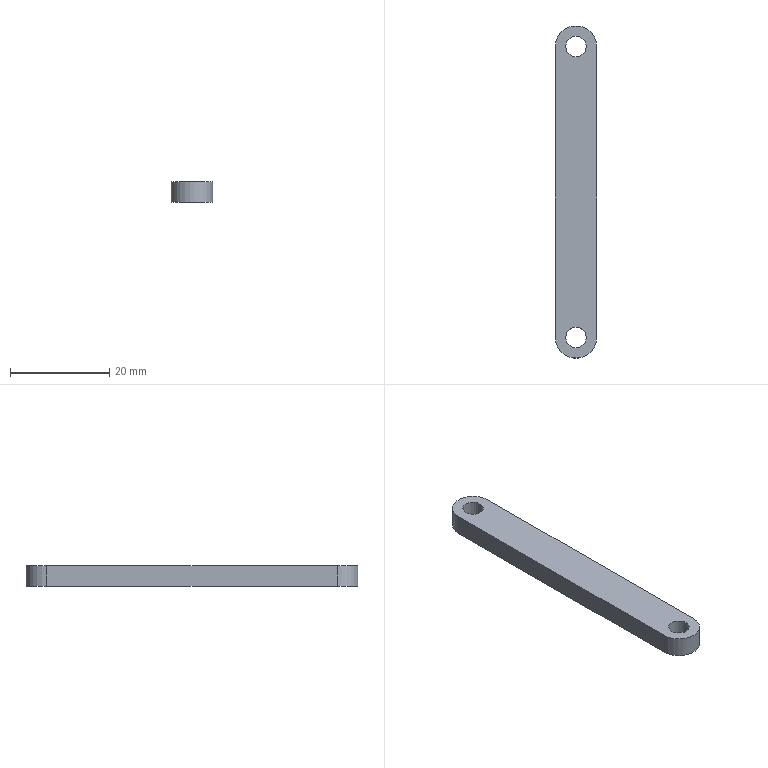Part | SolidWorks | features Extrusion 1, Scale 1 | 1 solid | 10 faces | box 8.32 x 66.82 x 4.134 mm | volume 2126 mm3 | cylinder 6 | plane 4 | commonest cylinder face diameters 4.134 x4 8.32 x2
STEP:
#1=CARTESIAN_POINT('',(-2.067,58.5,4.134));
#2=VERTEX_POINT('',#1);
#3=CARTESIAN_POINT('',(2.067,58.5,4.134));
#4=VERTEX_POINT('',#3);
#5=CARTESIAN_POINT('',(0.,58.5,4.134));
#6=DIRECTION('',(0.,0.,1.));
#7=DIRECTION('',(1.,0.,0.));
#8=AXIS2_PLACEMENT_3D('',#5,#6,#7);
#9=CIRCLE('',#8,2.067);
#10=EDGE_CURVE('',#2,#4,#9,.T.);
#11=ORIENTED_EDGE('',*,*,#10,.T.);
#12=CARTESIAN_POINT('',(2.067,58.5,0.));
#13=VERTEX_POINT('',#12);
#14=CARTESIAN_POINT('',(2.067,58.5,4.134));
#15=DIRECTION('',(0.,0.,-1.));
#16=VECTOR('',#15,1000.);
#17=LINE('',#14,#16);
#18=EDGE_CURVE('',#4,#13,#17,.T.);
#19=ORIENTED_EDGE('',*,*,#18,.T.);
#20=CARTESIAN_POINT('',(-2.067,58.5,0.));
#21=VERTEX_POINT('',#20);
#22=CARTESIAN_POINT('',(0.,58.5,0.));
#23=DIRECTION('',(0.,0.,1.));
#24=DIRECTION('',(1.,0.,0.));
#25=AXIS2_PLACEMENT_3D('',#22,#23,#24);
#26=CIRCLE('',#25,2.067);
#27=EDGE_CURVE('',#21,#13,#26,.T.);
#28=ORIENTED_EDGE('',*,*,#27,.F.);
#29=CARTESIAN_POINT('',(-2.067,58.5,4.134));
#30=DIRECTION('',(0.,0.,-1.));
#31=VECTOR('',#30,1000.);
#32=LINE('',#29,#31);
#33=EDGE_CURVE('',#2,#21,#32,.T.);
#34=ORIENTED_EDGE('',*,*,#33,.F.);
#35=EDGE_LOOP('',(#11,#19,#28,#34));
#36=FACE_OUTER_BOUND('',#35,.T.);
#37=CARTESIAN_POINT('',(0.,58.5,4.134));
#38=DIRECTION('',(0.,0.,-1.));
#39=DIRECTION('',(-1.,0.,0.));
#40=AXIS2_PLACEMENT_3D('',#37,#38,#39);
#41=CYLINDRICAL_SURFACE('',#40,2.067);
#42=ADVANCED_FACE('',(#36),#41,.F.);
#43=CARTESIAN_POINT('',(-2.067,0.,4.134));
#44=VERTEX_POINT('',#43);
#45=CARTESIAN_POINT('',(2.067,0.,4.134));
#46=VERTEX_POINT('',#45);
#47=CARTESIAN_POINT('',(0.,0.,4.134));
#48=DIRECTION('',(0.,0.,1.));
#49=DIRECTION('',(1.,0.,0.));
#50=AXIS2_PLACEMENT_3D('',#47,#48,#49);
#51=CIRCLE('',#50,2.067);
#52=EDGE_CURVE('',#44,#46,#51,.T.);
#53=ORIENTED_EDGE('',*,*,#52,.T.);
#54=CARTESIAN_POINT('',(2.067,0.,0.));
#55=VERTEX_POINT('',#54);
#56=CARTESIAN_POINT('',(2.067,0.,4.134));
#57=DIRECTION('',(0.,0.,-1.));
#58=VECTOR('',#57,1000.);
#59=LINE('',#56,#58);
#60=EDGE_CURVE('',#46,#55,#59,.T.);
#61=ORIENTED_EDGE('',*,*,#60,.T.);
#62=CARTESIAN_POINT('',(-2.067,0.,0.));
#63=VERTEX_POINT('',#62);
#64=CARTESIAN_POINT('',(0.,0.,0.));
#65=DIRECTION('',(0.,0.,1.));
#66=DIRECTION('',(1.,0.,0.));
#67=AXIS2_PLACEMENT_3D('',#64,#65,#66);
#68=CIRCLE('',#67,2.067);
#69=EDGE_CURVE('',#63,#55,#68,.T.);
#70=ORIENTED_EDGE('',*,*,#69,.F.);
#71=CARTESIAN_POINT('',(-2.067,0.,4.134));
#72=DIRECTION('',(0.,0.,-1.));
#73=VECTOR('',#72,1000.);
#74=LINE('',#71,#73);
#75=EDGE_CURVE('',#44,#63,#74,.T.);
#76=ORIENTED_EDGE('',*,*,#75,.F.);
#77=EDGE_LOOP('',(#53,#61,#70,#76));
#78=FACE_OUTER_BOUND('',#77,.T.);
#79=CARTESIAN_POINT('',(0.,0.,4.134));
#80=DIRECTION('',(0.,0.,-1.));
#81=DIRECTION('',(-1.,0.,0.));
#82=AXIS2_PLACEMENT_3D('',#79,#80,#81);
#83=CYLINDRICAL_SURFACE('',#82,2.067);
#84=ADVANCED_FACE('',(#78),#83,.F.);
#85=ORIENTED_EDGE('',*,*,#52,.F.);
#86=CARTESIAN_POINT('',(0.,0.,4.134));
#87=DIRECTION('',(0.,0.,1.));
#88=DIRECTION('',(1.,0.,0.));
#89=AXIS2_PLACEMENT_3D('',#86,#87,#88);
#90=CIRCLE('',#89,2.067);
#91=EDGE_CURVE('',#46,#44,#90,.T.);
#92=ORIENTED_EDGE('',*,*,#91,.F.);
#93=EDGE_LOOP('',(#85,#92));
#94=FACE_BOUND('',#93,.T.);
#95=CARTESIAN_POINT('',(-4.16,0.,4.134));
#96=VERTEX_POINT('',#95);
#97=CARTESIAN_POINT('',(4.16,0.,4.134));
#98=VERTEX_POINT('',#97);
#99=CARTESIAN_POINT('',(0.,0.,4.134));
#100=DIRECTION('',(0.,0.,1.));
#101=DIRECTION('',(1.,0.,0.));
#102=AXIS2_PLACEMENT_3D('',#99,#100,#101);
#103=CIRCLE('',#102,4.16);
#104=EDGE_CURVE('',#96,#98,#103,.T.);
#105=ORIENTED_EDGE('',*,*,#104,.T.);
#106=CARTESIAN_POINT('',(4.16,58.5,4.134));
#107=VERTEX_POINT('',#106);
#108=CARTESIAN_POINT('',(4.16,0.,4.134));
#109=DIRECTION('',(0.,1.,0.));
#110=VECTOR('',#109,1000.);
#111=LINE('',#108,#110);
#112=EDGE_CURVE('',#98,#107,#111,.T.);
#113=ORIENTED_EDGE('',*,*,#112,.T.);
#114=CARTESIAN_POINT('',(-4.16,58.5,4.134));
#115=VERTEX_POINT('',#114);
#116=CARTESIAN_POINT('',(0.,58.5,4.134));
#117=DIRECTION('',(0.,0.,1.));
#118=DIRECTION('',(1.,0.,0.));
#119=AXIS2_PLACEMENT_3D('',#116,#117,#118);
#120=CIRCLE('',#119,4.16);
#121=EDGE_CURVE('',#107,#115,#120,.T.);
#122=ORIENTED_EDGE('',*,*,#121,.T.);
#123=CARTESIAN_POINT('',(-4.16,0.,4.134));
#124=DIRECTION('',(0.,-1.,0.));
#125=VECTOR('',#124,1000.);
#126=LINE('',#123,#125);
#127=EDGE_CURVE('',#115,#96,#126,.T.);
#128=ORIENTED_EDGE('',*,*,#127,.T.);
#129=EDGE_LOOP('',(#105,#113,#122,#128));
#130=FACE_OUTER_BOUND('',#129,.T.);
#131=ORIENTED_EDGE('',*,*,#10,.F.);
#132=CARTESIAN_POINT('',(0.,58.5,4.134));
#133=DIRECTION('',(0.,0.,1.));
#134=DIRECTION('',(1.,0.,0.));
#135=AXIS2_PLACEMENT_3D('',#132,#133,#134);
#136=CIRCLE('',#135,2.067);
#137=EDGE_CURVE('',#4,#2,#136,.T.);
#138=ORIENTED_EDGE('',*,*,#137,.F.);
#139=EDGE_LOOP('',(#131,#138));
#140=FACE_BOUND('',#139,.T.);
#141=CARTESIAN_POINT('',(0.,0.,4.134));
#142=DIRECTION('',(0.,0.,1.));
#143=DIRECTION('',(1.,0.,0.));
#144=AXIS2_PLACEMENT_3D('',#141,#142,#143);
#145=PLANE('',#144);
#146=ADVANCED_FACE('',(#94,#130,#140),#145,.T.);
#147=CARTESIAN_POINT('',(-4.16,0.,0.));
#148=VERTEX_POINT('',#147);
#149=CARTESIAN_POINT('',(4.16,0.,0.));
#150=VERTEX_POINT('',#149);
#151=CARTESIAN_POINT('',(0.,0.,0.));
#152=DIRECTION('',(0.,0.,1.));
#153=DIRECTION('',(1.,0.,0.));
#154=AXIS2_PLACEMENT_3D('',#151,#152,#153);
#155=CIRCLE('',#154,4.16);
#156=EDGE_CURVE('',#148,#150,#155,.T.);
#157=ORIENTED_EDGE('',*,*,#156,.F.);
#158=CARTESIAN_POINT('',(-4.16,58.5,0.));
#159=VERTEX_POINT('',#158);
#160=CARTESIAN_POINT('',(-4.16,0.,0.));
#161=DIRECTION('',(0.,-1.,0.));
#162=VECTOR('',#161,1000.);
#163=LINE('',#160,#162);
#164=EDGE_CURVE('',#159,#148,#163,.T.);
#165=ORIENTED_EDGE('',*,*,#164,.F.);
#166=CARTESIAN_POINT('',(4.16,58.5,0.));
#167=VERTEX_POINT('',#166);
#168=CARTESIAN_POINT('',(0.,58.5,0.));
#169=DIRECTION('',(0.,0.,1.));
#170=DIRECTION('',(1.,0.,0.));
#171=AXIS2_PLACEMENT_3D('',#168,#169,#170);
#172=CIRCLE('',#171,4.16);
#173=EDGE_CURVE('',#167,#159,#172,.T.);
#174=ORIENTED_EDGE('',*,*,#173,.F.);
#175=CARTESIAN_POINT('',(4.16,0.,0.));
#176=DIRECTION('',(0.,1.,0.));
#177=VECTOR('',#176,1000.);
#178=LINE('',#175,#177);
#179=EDGE_CURVE('',#150,#167,#178,.T.);
#180=ORIENTED_EDGE('',*,*,#179,.F.);
#181=EDGE_LOOP('',(#157,#165,#174,#180));
#182=FACE_OUTER_BOUND('',#181,.T.);
#183=ORIENTED_EDGE('',*,*,#69,.T.);
#184=CARTESIAN_POINT('',(0.,0.,0.));
#185=DIRECTION('',(0.,0.,1.));
#186=DIRECTION('',(1.,0.,0.));
#187=AXIS2_PLACEMENT_3D('',#184,#185,#186);
#188=CIRCLE('',#187,2.067);
#189=EDGE_CURVE('',#55,#63,#188,.T.);
#190=ORIENTED_EDGE('',*,*,#189,.T.);
#191=EDGE_LOOP('',(#183,#190));
#192=FACE_BOUND('',#191,.T.);
#193=ORIENTED_EDGE('',*,*,#27,.T.);
#194=CARTESIAN_POINT('',(0.,58.5,0.));
#195=DIRECTION('',(0.,0.,1.));
#196=DIRECTION('',(1.,0.,0.));
#197=AXIS2_PLACEMENT_3D('',#194,#195,#196);
#198=CIRCLE('',#197,2.067);
#199=EDGE_CURVE('',#13,#21,#198,.T.);
#200=ORIENTED_EDGE('',*,*,#199,.T.);
#201=EDGE_LOOP('',(#193,#200));
#202=FACE_BOUND('',#201,.T.);
#203=CARTESIAN_POINT('',(0.,0.,0.));
#204=DIRECTION('',(0.,0.,1.));
#205=DIRECTION('',(1.,0.,0.));
#206=AXIS2_PLACEMENT_3D('',#203,#204,#205);
#207=PLANE('',#206);
#208=ADVANCED_FACE('',(#182,#192,#202),#207,.F.);
#209=ORIENTED_EDGE('',*,*,#156,.T.);
#210=CARTESIAN_POINT('',(4.16,0.,4.134));
#211=DIRECTION('',(0.,0.,-1.));
#212=VECTOR('',#211,1000.);
#213=LINE('',#210,#212);
#214=EDGE_CURVE('',#98,#150,#213,.T.);
#215=ORIENTED_EDGE('',*,*,#214,.F.);
#216=ORIENTED_EDGE('',*,*,#104,.F.);
#217=CARTESIAN_POINT('',(-4.16,0.,4.134));
#218=DIRECTION('',(0.,0.,-1.));
#219=VECTOR('',#218,1000.);
#220=LINE('',#217,#219);
#221=EDGE_CURVE('',#96,#148,#220,.T.);
#222=ORIENTED_EDGE('',*,*,#221,.T.);
#223=EDGE_LOOP('',(#209,#215,#216,#222));
#224=FACE_OUTER_BOUND('',#223,.T.);
#225=CARTESIAN_POINT('',(0.,0.,4.134));
#226=DIRECTION('',(0.,0.,-1.));
#227=DIRECTION('',(-1.,0.,0.));
#228=AXIS2_PLACEMENT_3D('',#225,#226,#227);
#229=CYLINDRICAL_SURFACE('',#228,4.16);
#230=ADVANCED_FACE('',(#224),#229,.T.);
#231=ORIENTED_EDGE('',*,*,#179,.T.);
#232=CARTESIAN_POINT('',(4.16,58.5,4.134));
#233=DIRECTION('',(0.,0.,-1.));
#234=VECTOR('',#233,1000.);
#235=LINE('',#232,#234);
#236=EDGE_CURVE('',#107,#167,#235,.T.);
#237=ORIENTED_EDGE('',*,*,#236,.F.);
#238=ORIENTED_EDGE('',*,*,#112,.F.);
#239=ORIENTED_EDGE('',*,*,#214,.T.);
#240=EDGE_LOOP('',(#231,#237,#238,#239));
#241=FACE_OUTER_BOUND('',#240,.T.);
#242=CARTESIAN_POINT('',(4.16,0.,4.134));
#243=DIRECTION('',(-1.,0.,0.));
#244=DIRECTION('',(0.,0.,1.));
#245=AXIS2_PLACEMENT_3D('',#242,#243,#244);
#246=PLANE('',#245);
#247=ADVANCED_FACE('',(#241),#246,.F.);
#248=ORIENTED_EDGE('',*,*,#173,.T.);
#249=CARTESIAN_POINT('',(-4.16,58.5,4.134));
#250=DIRECTION('',(0.,0.,-1.));
#251=VECTOR('',#250,1000.);
#252=LINE('',#249,#251);
#253=EDGE_CURVE('',#115,#159,#252,.T.);
#254=ORIENTED_EDGE('',*,*,#253,.F.);
#255=ORIENTED_EDGE('',*,*,#121,.F.);
#256=ORIENTED_EDGE('',*,*,#236,.T.);
#257=EDGE_LOOP('',(#248,#254,#255,#256));
#258=FACE_OUTER_BOUND('',#257,.T.);
#259=CARTESIAN_POINT('',(0.,58.5,4.134));
#260=DIRECTION('',(0.,0.,-1.));
#261=DIRECTION('',(-1.,0.,0.));
#262=AXIS2_PLACEMENT_3D('',#259,#260,#261);
#263=CYLINDRICAL_SURFACE('',#262,4.16);
#264=ADVANCED_FACE('',(#258),#263,.T.);
#265=ORIENTED_EDGE('',*,*,#164,.T.);
#266=ORIENTED_EDGE('',*,*,#221,.F.);
#267=ORIENTED_EDGE('',*,*,#127,.F.);
#268=ORIENTED_EDGE('',*,*,#253,.T.);
#269=EDGE_LOOP('',(#265,#266,#267,#268));
#270=FACE_OUTER_BOUND('',#269,.T.);
#271=CARTESIAN_POINT('',(-4.16,0.,4.134));
#272=DIRECTION('',(1.,0.,0.));
#273=DIRECTION('',(0.,0.,-1.));
#274=AXIS2_PLACEMENT_3D('',#271,#272,#273);
#275=PLANE('',#274);
#276=ADVANCED_FACE('',(#270),#275,.F.);
#277=ORIENTED_EDGE('',*,*,#60,.F.);
#278=ORIENTED_EDGE('',*,*,#91,.T.);
#279=ORIENTED_EDGE('',*,*,#75,.T.);
#280=ORIENTED_EDGE('',*,*,#189,.F.);
#281=EDGE_LOOP('',(#277,#278,#279,#280));
#282=FACE_OUTER_BOUND('',#281,.T.);
#283=CARTESIAN_POINT('',(0.,0.,4.134));
#284=DIRECTION('',(0.,0.,-1.));
#285=DIRECTION('',(-1.,0.,0.));
#286=AXIS2_PLACEMENT_3D('',#283,#284,#285);
#287=CYLINDRICAL_SURFACE('',#286,2.067);
#288=ADVANCED_FACE('',(#282),#287,.F.);
#289=ORIENTED_EDGE('',*,*,#18,.F.);
#290=ORIENTED_EDGE('',*,*,#137,.T.);
#291=ORIENTED_EDGE('',*,*,#33,.T.);
#292=ORIENTED_EDGE('',*,*,#199,.F.);
#293=EDGE_LOOP('',(#289,#290,#291,#292));
#294=FACE_OUTER_BOUND('',#293,.T.);
#295=CARTESIAN_POINT('',(0.,58.5,4.134));
#296=DIRECTION('',(0.,0.,-1.));
#297=DIRECTION('',(-1.,0.,0.));
#298=AXIS2_PLACEMENT_3D('',#295,#296,#297);
#299=CYLINDRICAL_SURFACE('',#298,2.067);
#300=ADVANCED_FACE('',(#294),#299,.F.);
#301=CLOSED_SHELL('',(#42,#84,#146,#208,#230,#247,#264,#276,#288,#300));
#302=MANIFOLD_SOLID_BREP('',#301);
#303=CARTESIAN_POINT('',(0.,0.,0.));
#304=DIRECTION('',(0.,0.,1.));
#305=DIRECTION('',(1.,0.,0.));
#306=AXIS2_PLACEMENT_3D('',#303,#304,#305);
#307=(LENGTH_UNIT()NAMED_UNIT(*)SI_UNIT(.MILLI.,.METRE.));
#308=UNCERTAINTY_MEASURE_WITH_UNIT(LENGTH_MEASURE(0.00001),#307,'','');
#309=(NAMED_UNIT(*)PLANE_ANGLE_UNIT()SI_UNIT($,.RADIAN.));
#310=(NAMED_UNIT(*)SI_UNIT($,.STERADIAN.)SOLID_ANGLE_UNIT());
#311=(GEOMETRIC_REPRESENTATION_CONTEXT(3)GLOBAL_UNCERTAINTY_ASSIGNED_CONTEXT((#308))GLOBAL_UNIT_ASSIGNED_CONTEXT((#307,#309,#310))REPRESENTATION_CONTEXT('',''));
#312=ADVANCED_BREP_SHAPE_REPRESENTATION('',(#302,#306),#311);